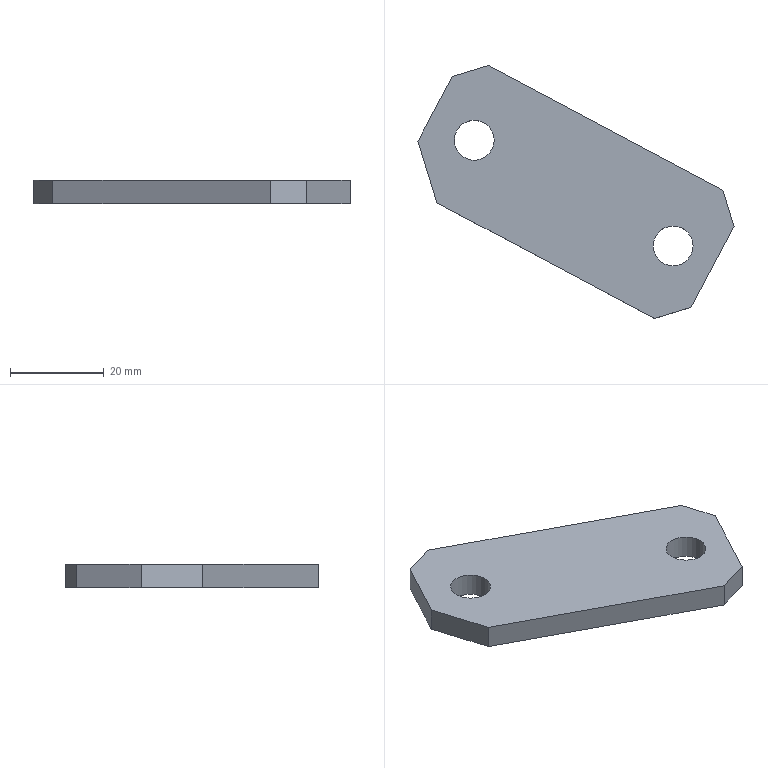Part | STEP file | gslz 2016.10.28-13_id1682_x_t | 1 solid | 12 faces | box 67.358 x 53.937 x 5 mm | volume 9493 mm3 | plane 10 | cylinder 2 | commonest cylinder face diameters 8.5 x2
STEP:
#1=CARTESIAN_POINT('',(0.,0.,0.));
#2=DIRECTION('',(0.,0.,1.));
#3=DIRECTION('',(1.,0.,0.));
#4=AXIS2_PLACEMENT_3D('',#1,#2,#3);
#5=CARTESIAN_POINT('',(446.195,-230.193,-94.));
#6=VERTEX_POINT('',#5);
#7=CARTESIAN_POINT('',(396.233,-203.628,-94.));
#8=VERTEX_POINT('',#7);
#9=CARTESIAN_POINT('',(-202.815,114.892,-94.));
#10=DIRECTION('',(-0.8829,0.4695,0.));
#11=VECTOR('',#10,1.);
#12=LINE('',#9,#11);
#13=CARTESIAN_POINT('',(-202.815,114.892,-99.));
#14=DIRECTION('',(0.4695,0.8829,0.));
#15=DIRECTION('',(-0.8829,0.4695,0.));
#16=AXIS2_PLACEMENT_3D('',#13,#14,#15);
#17=PLANE('',#16);
#18=CARTESIAN_POINT('',(0.,5.));
#19=DIRECTION('',(1.,0.));
#20=VECTOR('',#19,1.);
#21=LINE('',#18,#20);
#22=(GEOMETRIC_REPRESENTATION_CONTEXT(2)PARAMETRIC_REPRESENTATION_CONTEXT()REPRESENTATION_CONTEXT('',''));
#23=DEFINITIONAL_REPRESENTATION('',(#21),#22);
#24=PCURVE('',#17,#23);
#25=CARTESIAN_POINT('',(-224.645,73.835,-94.));
#26=DIRECTION('',(0.,0.,-1.));
#27=DIRECTION('',(-1.,0.,0.));
#28=AXIS2_PLACEMENT_3D('',#25,#26,#27);
#29=PLANE('',#28);
#30=CARTESIAN_POINT('',(-21.83,41.057));
#31=DIRECTION('',(0.8829,0.4695));
#32=VECTOR('',#31,1.);
#33=LINE('',#30,#32);
#34=(GEOMETRIC_REPRESENTATION_CONTEXT(2)PARAMETRIC_REPRESENTATION_CONTEXT()REPRESENTATION_CONTEXT('',''));
#35=DEFINITIONAL_REPRESENTATION('',(#33),#34);
#36=PCURVE('',#29,#35);
#37=SURFACE_CURVE('',#12,(#24,#36),.PCURVE_S1.);
#38=EDGE_CURVE('',#6,#8,#37,.T.);
#39=ORIENTED_EDGE('',*,*,#38,.F.);
#40=CARTESIAN_POINT('',(446.195,-230.193,-99.));
#41=VERTEX_POINT('',#40);
#42=CARTESIAN_POINT('',(446.195,-230.193,-99.));
#43=DIRECTION('',(0.,0.,-1.));
#44=VECTOR('',#43,1.);
#45=LINE('',#42,#44);
#46=CARTESIAN_POINT('',(-735.049,0.));
#47=DIRECTION('',(0.,-1.));
#48=VECTOR('',#47,1.);
#49=LINE('',#46,#48);
#50=(GEOMETRIC_REPRESENTATION_CONTEXT(2)PARAMETRIC_REPRESENTATION_CONTEXT()REPRESENTATION_CONTEXT('',''));
#51=DEFINITIONAL_REPRESENTATION('',(#49),#50);
#52=PCURVE('',#17,#51);
#53=CARTESIAN_POINT('',(448.615,-238.11,-99.));
#54=DIRECTION('',(-0.9563,-0.2924,0.));
#55=DIRECTION('',(0.,0.,1.));
#56=AXIS2_PLACEMENT_3D('',#53,#54,#55);
#57=PLANE('',#56);
#58=CARTESIAN_POINT('',(0.,8.278));
#59=DIRECTION('',(-1.,0.));
#60=VECTOR('',#59,1.);
#61=LINE('',#58,#60);
#62=(GEOMETRIC_REPRESENTATION_CONTEXT(2)PARAMETRIC_REPRESENTATION_CONTEXT()REPRESENTATION_CONTEXT('',''));
#63=DEFINITIONAL_REPRESENTATION('',(#61),#62);
#64=PCURVE('',#57,#63);
#65=SURFACE_CURVE('',#45,(#52,#64),.PCURVE_S1.);
#66=EDGE_CURVE('',#6,#41,#65,.T.);
#67=ORIENTED_EDGE('',*,*,#66,.T.);
#68=CARTESIAN_POINT('',(396.233,-203.628,-99.));
#69=VERTEX_POINT('',#68);
#70=CARTESIAN_POINT('',(-202.815,114.892,-99.));
#71=DIRECTION('',(-0.8829,0.4695,0.));
#72=VECTOR('',#71,1.);
#73=LINE('',#70,#72);
#74=CARTESIAN_POINT('',(0.,0.));
#75=DIRECTION('',(1.,0.));
#76=VECTOR('',#75,1.);
#77=LINE('',#74,#76);
#78=(GEOMETRIC_REPRESENTATION_CONTEXT(2)PARAMETRIC_REPRESENTATION_CONTEXT()REPRESENTATION_CONTEXT('',''));
#79=DEFINITIONAL_REPRESENTATION('',(#77),#78);
#80=PCURVE('',#17,#79);
#81=CARTESIAN_POINT('',(-224.645,73.835,-99.));
#82=DIRECTION('',(0.,0.,-1.));
#83=DIRECTION('',(-1.,0.,0.));
#84=AXIS2_PLACEMENT_3D('',#81,#82,#83);
#85=PLANE('',#84);
#86=CARTESIAN_POINT('',(-21.83,41.057));
#87=DIRECTION('',(0.8829,0.4695));
#88=VECTOR('',#87,1.);
#89=LINE('',#86,#88);
#90=(GEOMETRIC_REPRESENTATION_CONTEXT(2)PARAMETRIC_REPRESENTATION_CONTEXT()REPRESENTATION_CONTEXT('',''));
#91=DEFINITIONAL_REPRESENTATION('',(#89),#90);
#92=PCURVE('',#85,#91);
#93=SURFACE_CURVE('',#73,(#80,#92),.PCURVE_S1.);
#94=EDGE_CURVE('',#41,#69,#93,.T.);
#95=ORIENTED_EDGE('',*,*,#94,.T.);
#96=CARTESIAN_POINT('',(396.233,-203.628,-99.));
#97=DIRECTION('',(0.,0.,1.));
#98=VECTOR('',#97,1.);
#99=LINE('',#96,#98);
#100=CARTESIAN_POINT('',(-678.463,0.));
#101=DIRECTION('',(0.,1.));
#102=VECTOR('',#101,1.);
#103=LINE('',#100,#102);
#104=(GEOMETRIC_REPRESENTATION_CONTEXT(2)PARAMETRIC_REPRESENTATION_CONTEXT()REPRESENTATION_CONTEXT('',''));
#105=DEFINITIONAL_REPRESENTATION('',(#103),#104);
#106=PCURVE('',#17,#105);
#107=CARTESIAN_POINT('',(396.431,-203.567,-99.));
#108=DIRECTION('',(-0.2924,0.9563,0.));
#109=DIRECTION('',(0.,0.,-1.));
#110=AXIS2_PLACEMENT_3D('',#107,#108,#109);
#111=PLANE('',#110);
#112=CARTESIAN_POINT('',(0.,0.2071));
#113=DIRECTION('',(-1.,0.));
#114=VECTOR('',#113,1.);
#115=LINE('',#112,#114);
#116=(GEOMETRIC_REPRESENTATION_CONTEXT(2)PARAMETRIC_REPRESENTATION_CONTEXT()REPRESENTATION_CONTEXT('',''));
#117=DEFINITIONAL_REPRESENTATION('',(#115),#116);
#118=PCURVE('',#111,#117);
#119=SURFACE_CURVE('',#99,(#106,#118),.PCURVE_S1.);
#120=EDGE_CURVE('',#69,#8,#119,.T.);
#121=ORIENTED_EDGE('',*,*,#120,.T.);
#122=EDGE_LOOP('',(#39,#67,#95,#121));
#123=FACE_BOUND('',#122,.T.);
#124=ADVANCED_FACE('',(#123),#17,.T.);
#125=CARTESIAN_POINT('',(439.36,-255.205,-94.));
#126=VERTEX_POINT('',#125);
#127=CARTESIAN_POINT('',(448.555,-237.912,-94.));
#128=VERTEX_POINT('',#127);
#129=CARTESIAN_POINT('',(429.404,-273.93,-94.));
#130=DIRECTION('',(0.4695,0.8829,0.));
#131=VECTOR('',#130,1.);
#132=LINE('',#129,#131);
#133=CARTESIAN_POINT('',(429.404,-273.93,-99.));
#134=DIRECTION('',(0.8829,-0.4695,0.));
#135=DIRECTION('',(0.4695,0.8829,0.));
#136=AXIS2_PLACEMENT_3D('',#133,#134,#135);
#137=PLANE('',#136);
#138=CARTESIAN_POINT('',(0.,5.));
#139=DIRECTION('',(1.,0.));
#140=VECTOR('',#139,1.);
#141=LINE('',#138,#140);
#142=(GEOMETRIC_REPRESENTATION_CONTEXT(2)PARAMETRIC_REPRESENTATION_CONTEXT()REPRESENTATION_CONTEXT('',''));
#143=DEFINITIONAL_REPRESENTATION('',(#141),#142);
#144=PCURVE('',#137,#143);
#145=CARTESIAN_POINT('',(-654.049,-347.764));
#146=DIRECTION('',(-0.4695,0.8829));
#147=VECTOR('',#146,1.);
#148=LINE('',#145,#147);
#149=(GEOMETRIC_REPRESENTATION_CONTEXT(2)PARAMETRIC_REPRESENTATION_CONTEXT()REPRESENTATION_CONTEXT('',''));
#150=DEFINITIONAL_REPRESENTATION('',(#148),#149);
#151=PCURVE('',#29,#150);
#152=SURFACE_CURVE('',#132,(#144,#151),.PCURVE_S1.);
#153=EDGE_CURVE('',#126,#128,#152,.T.);
#154=ORIENTED_EDGE('',*,*,#153,.F.);
#155=CARTESIAN_POINT('',(439.36,-255.205,-99.));
#156=VERTEX_POINT('',#155);
#157=CARTESIAN_POINT('',(439.36,-255.205,-99.));
#158=DIRECTION('',(0.,0.,-1.));
#159=VECTOR('',#158,1.);
#160=LINE('',#157,#159);
#161=CARTESIAN_POINT('',(21.207,0.));
#162=DIRECTION('',(0.,-1.));
#163=VECTOR('',#162,1.);
#164=LINE('',#161,#163);
#165=(GEOMETRIC_REPRESENTATION_CONTEXT(2)PARAMETRIC_REPRESENTATION_CONTEXT()REPRESENTATION_CONTEXT('',''));
#166=DEFINITIONAL_REPRESENTATION('',(#164),#165);
#167=PCURVE('',#137,#166);
#168=CARTESIAN_POINT('',(431.443,-257.625,-99.));
#169=DIRECTION('',(0.2924,-0.9563,0.));
#170=DIRECTION('',(0.,0.,-1.));
#171=AXIS2_PLACEMENT_3D('',#168,#169,#170);
#172=PLANE('',#171);
#173=CARTESIAN_POINT('',(0.,8.278));
#174=DIRECTION('',(1.,0.));
#175=VECTOR('',#174,1.);
#176=LINE('',#173,#175);
#177=(GEOMETRIC_REPRESENTATION_CONTEXT(2)PARAMETRIC_REPRESENTATION_CONTEXT()REPRESENTATION_CONTEXT('',''));
#178=DEFINITIONAL_REPRESENTATION('',(#176),#177);
#179=PCURVE('',#172,#178);
#180=SURFACE_CURVE('',#160,(#167,#179),.PCURVE_S1.);
#181=EDGE_CURVE('',#126,#156,#180,.T.);
#182=ORIENTED_EDGE('',*,*,#181,.T.);
#183=CARTESIAN_POINT('',(448.555,-237.912,-99.));
#184=VERTEX_POINT('',#183);
#185=CARTESIAN_POINT('',(429.404,-273.93,-99.));
#186=DIRECTION('',(0.4695,0.8829,0.));
#187=VECTOR('',#186,1.);
#188=LINE('',#185,#187);
#189=CARTESIAN_POINT('',(0.,0.));
#190=DIRECTION('',(1.,0.));
#191=VECTOR('',#190,1.);
#192=LINE('',#189,#191);
#193=(GEOMETRIC_REPRESENTATION_CONTEXT(2)PARAMETRIC_REPRESENTATION_CONTEXT()REPRESENTATION_CONTEXT('',''));
#194=DEFINITIONAL_REPRESENTATION('',(#192),#193);
#195=PCURVE('',#137,#194);
#196=CARTESIAN_POINT('',(-654.049,-347.764));
#197=DIRECTION('',(-0.4695,0.8829));
#198=VECTOR('',#197,1.);
#199=LINE('',#196,#198);
#200=(GEOMETRIC_REPRESENTATION_CONTEXT(2)PARAMETRIC_REPRESENTATION_CONTEXT()REPRESENTATION_CONTEXT('',''));
#201=DEFINITIONAL_REPRESENTATION('',(#199),#200);
#202=PCURVE('',#85,#201);
#203=SURFACE_CURVE('',#188,(#195,#202),.PCURVE_S1.);
#204=EDGE_CURVE('',#156,#184,#203,.T.);
#205=ORIENTED_EDGE('',*,*,#204,.T.);
#206=CARTESIAN_POINT('',(448.555,-237.912,-99.));
#207=DIRECTION('',(0.,0.,1.));
#208=VECTOR('',#207,1.);
#209=LINE('',#206,#208);
#210=CARTESIAN_POINT('',(40.793,0.));
#211=DIRECTION('',(0.,1.));
#212=VECTOR('',#211,1.);
#213=LINE('',#210,#212);
#214=(GEOMETRIC_REPRESENTATION_CONTEXT(2)PARAMETRIC_REPRESENTATION_CONTEXT()REPRESENTATION_CONTEXT('',''));
#215=DEFINITIONAL_REPRESENTATION('',(#213),#214);
#216=PCURVE('',#137,#215);
#217=CARTESIAN_POINT('',(0.,0.2071));
#218=DIRECTION('',(1.,0.));
#219=VECTOR('',#218,1.);
#220=LINE('',#217,#219);
#221=(GEOMETRIC_REPRESENTATION_CONTEXT(2)PARAMETRIC_REPRESENTATION_CONTEXT()REPRESENTATION_CONTEXT('',''));
#222=DEFINITIONAL_REPRESENTATION('',(#220),#221);
#223=PCURVE('',#57,#222);
#224=SURFACE_CURVE('',#209,(#216,#223),.PCURVE_S1.);
#225=EDGE_CURVE('',#184,#128,#224,.T.);
#226=ORIENTED_EDGE('',*,*,#225,.T.);
#227=EDGE_LOOP('',(#154,#182,#205,#226));
#228=FACE_BOUND('',#227,.T.);
#229=ADVANCED_FACE('',(#228),#137,.T.);
#230=CARTESIAN_POINT('',(431.641,-257.564,-94.));
#231=VERTEX_POINT('',#230);
#232=CARTESIAN_POINT('',(385.211,-232.877,-94.));
#233=VERTEX_POINT('',#232);
#234=CARTESIAN_POINT('',(-217.368,87.52,-94.));
#235=DIRECTION('',(-0.8829,0.4695,0.));
#236=VECTOR('',#235,1.);
#237=LINE('',#234,#236);
#238=CARTESIAN_POINT('',(-217.368,87.52,-99.));
#239=DIRECTION('',(0.4695,0.8829,0.));
#240=DIRECTION('',(-0.8829,0.4695,0.));
#241=AXIS2_PLACEMENT_3D('',#238,#239,#240);
#242=PLANE('',#241);
#243=CARTESIAN_POINT('',(0.,5.));
#244=DIRECTION('',(1.,0.));
#245=VECTOR('',#244,1.);
#246=LINE('',#243,#245);
#247=(GEOMETRIC_REPRESENTATION_CONTEXT(2)PARAMETRIC_REPRESENTATION_CONTEXT()REPRESENTATION_CONTEXT('',''));
#248=DEFINITIONAL_REPRESENTATION('',(#246),#247);
#249=PCURVE('',#242,#248);
#250=CARTESIAN_POINT('',(-7.277,13.686));
#251=DIRECTION('',(0.8829,0.4695));
#252=VECTOR('',#251,1.);
#253=LINE('',#250,#252);
#254=(GEOMETRIC_REPRESENTATION_CONTEXT(2)PARAMETRIC_REPRESENTATION_CONTEXT()REPRESENTATION_CONTEXT('',''));
#255=DEFINITIONAL_REPRESENTATION('',(#253),#254);
#256=PCURVE('',#29,#255);
#257=SURFACE_CURVE('',#237,(#249,#256),.PCURVE_S1.);
#258=EDGE_CURVE('',#231,#233,#257,.T.);
#259=ORIENTED_EDGE('',*,*,#258,.T.);
#260=CARTESIAN_POINT('',(385.211,-232.877,-99.));
#261=VERTEX_POINT('',#260);
#262=CARTESIAN_POINT('',(385.211,-232.877,-99.));
#263=DIRECTION('',(0.,0.,-1.));
#264=VECTOR('',#263,1.);
#265=LINE('',#262,#264);
#266=CARTESIAN_POINT('',(-682.463,0.));
#267=DIRECTION('',(0.,-1.));
#268=VECTOR('',#267,1.);
#269=LINE('',#266,#268);
#270=(GEOMETRIC_REPRESENTATION_CONTEXT(2)PARAMETRIC_REPRESENTATION_CONTEXT()REPRESENTATION_CONTEXT('',''));
#271=DEFINITIONAL_REPRESENTATION('',(#269),#270);
#272=PCURVE('',#242,#271);
#273=CARTESIAN_POINT('',(381.137,-219.551,-99.));
#274=DIRECTION('',(0.9563,0.2924,0.));
#275=DIRECTION('',(0.,0.,1.));
#276=AXIS2_PLACEMENT_3D('',#273,#274,#275);
#277=PLANE('',#276);
#278=CARTESIAN_POINT('',(0.,13.935));
#279=DIRECTION('',(-1.,0.));
#280=VECTOR('',#279,1.);
#281=LINE('',#278,#280);
#282=(GEOMETRIC_REPRESENTATION_CONTEXT(2)PARAMETRIC_REPRESENTATION_CONTEXT()REPRESENTATION_CONTEXT('',''));
#283=DEFINITIONAL_REPRESENTATION('',(#281),#282);
#284=PCURVE('',#277,#283);
#285=SURFACE_CURVE('',#265,(#272,#284),.PCURVE_S1.);
#286=EDGE_CURVE('',#233,#261,#285,.T.);
#287=ORIENTED_EDGE('',*,*,#286,.T.);
#288=CARTESIAN_POINT('',(431.641,-257.564,-99.));
#289=VERTEX_POINT('',#288);
#290=CARTESIAN_POINT('',(-217.368,87.52,-99.));
#291=DIRECTION('',(-0.8829,0.4695,0.));
#292=VECTOR('',#291,1.);
#293=LINE('',#290,#292);
#294=CARTESIAN_POINT('',(0.,0.));
#295=DIRECTION('',(1.,0.));
#296=VECTOR('',#295,1.);
#297=LINE('',#294,#296);
#298=(GEOMETRIC_REPRESENTATION_CONTEXT(2)PARAMETRIC_REPRESENTATION_CONTEXT()REPRESENTATION_CONTEXT('',''));
#299=DEFINITIONAL_REPRESENTATION('',(#297),#298);
#300=PCURVE('',#242,#299);
#301=CARTESIAN_POINT('',(-7.277,13.686));
#302=DIRECTION('',(0.8829,0.4695));
#303=VECTOR('',#302,1.);
#304=LINE('',#301,#303);
#305=(GEOMETRIC_REPRESENTATION_CONTEXT(2)PARAMETRIC_REPRESENTATION_CONTEXT()REPRESENTATION_CONTEXT('',''));
#306=DEFINITIONAL_REPRESENTATION('',(#304),#305);
#307=PCURVE('',#85,#306);
#308=SURFACE_CURVE('',#293,(#300,#307),.PCURVE_S1.);
#309=EDGE_CURVE('',#289,#261,#308,.T.);
#310=ORIENTED_EDGE('',*,*,#309,.F.);
#311=CARTESIAN_POINT('',(431.641,-257.564,-99.));
#312=DIRECTION('',(0.,0.,1.));
#313=VECTOR('',#312,1.);
#314=LINE('',#311,#313);
#315=CARTESIAN_POINT('',(-735.049,0.));
#316=DIRECTION('',(0.,1.));
#317=VECTOR('',#316,1.);
#318=LINE('',#315,#317);
#319=(GEOMETRIC_REPRESENTATION_CONTEXT(2)PARAMETRIC_REPRESENTATION_CONTEXT()REPRESENTATION_CONTEXT('',''));
#320=DEFINITIONAL_REPRESENTATION('',(#318),#319);
#321=PCURVE('',#242,#320);
#322=CARTESIAN_POINT('',(0.,0.2071));
#323=DIRECTION('',(-1.,0.));
#324=VECTOR('',#323,1.);
#325=LINE('',#322,#324);
#326=(GEOMETRIC_REPRESENTATION_CONTEXT(2)PARAMETRIC_REPRESENTATION_CONTEXT()REPRESENTATION_CONTEXT('',''));
#327=DEFINITIONAL_REPRESENTATION('',(#325),#326);
#328=PCURVE('',#172,#327);
#329=SURFACE_CURVE('',#314,(#321,#328),.PCURVE_S1.);
#330=EDGE_CURVE('',#289,#231,#329,.T.);
#331=ORIENTED_EDGE('',*,*,#330,.T.);
#332=EDGE_LOOP('',(#259,#287,#310,#331));
#333=FACE_BOUND('',#332,.T.);
#334=ADVANCED_FACE('',(#333),#242,.F.);
#335=CARTESIAN_POINT('',(431.319,-242.098,-99.));
#336=VERTEX_POINT('',#335);
#337=CARTESIAN_POINT('',(435.569,-242.098,-99.));
#338=DIRECTION('',(0.,0.,-1.));
#339=DIRECTION('',(-1.,0.,0.));
#340=AXIS2_PLACEMENT_3D('',#337,#338,#339);
#341=CIRCLE('',#340,4.25);
#342=CARTESIAN_POINT('',(435.569,-242.098,-99.));
#343=DIRECTION('',(0.,0.,1.));
#344=DIRECTION('',(1.,0.,0.));
#345=AXIS2_PLACEMENT_3D('',#342,#343,#344);
#346=CYLINDRICAL_SURFACE('',#345,4.25);
#347=CARTESIAN_POINT('',(9.425,0.));
#348=DIRECTION('',(-1.,0.));
#349=VECTOR('',#348,1.);
#350=LINE('',#347,#349);
#351=(GEOMETRIC_REPRESENTATION_CONTEXT(2)PARAMETRIC_REPRESENTATION_CONTEXT()REPRESENTATION_CONTEXT('',''));
#352=DEFINITIONAL_REPRESENTATION('',(#350),#351);
#353=PCURVE('',#346,#352);
#354=CARTESIAN_POINT('',(-660.215,-315.933));
#355=DIRECTION('',(1.,0.));
#356=AXIS2_PLACEMENT_2D('',#354,#355);
#357=CIRCLE('',#356,4.25);
#358=(GEOMETRIC_REPRESENTATION_CONTEXT(2)PARAMETRIC_REPRESENTATION_CONTEXT()REPRESENTATION_CONTEXT('',''));
#359=DEFINITIONAL_REPRESENTATION('',(#357),#358);
#360=PCURVE('',#85,#359);
#361=SURFACE_CURVE('',#341,(#353,#360),.PCURVE_S1.);
#362=EDGE_CURVE('',#336,#336,#361,.T.);
#363=ORIENTED_EDGE('',*,*,#362,.F.);
#364=CARTESIAN_POINT('',(431.319,-242.098,-94.));
#365=VERTEX_POINT('',#364);
#366=CARTESIAN_POINT('',(431.319,-242.098,-99.));
#367=CARTESIAN_POINT('',(431.319,-242.098,-94.));
#368=B_SPLINE_CURVE_WITH_KNOTS('',1,(#366,#367),.UNSPECIFIED.,.F.,.F.,(2,2),(0.,5.),.PIECEWISE_BEZIER_KNOTS.);
#369=CARTESIAN_POINT('',(9.425,0.));
#370=DIRECTION('',(0.,1.));
#371=VECTOR('',#370,1.);
#372=LINE('',#369,#371);
#373=(GEOMETRIC_REPRESENTATION_CONTEXT(2)PARAMETRIC_REPRESENTATION_CONTEXT()REPRESENTATION_CONTEXT('',''));
#374=DEFINITIONAL_REPRESENTATION('',(#372),#373);
#375=PCURVE('',#346,#374);
#376=CARTESIAN_POINT('',(3.142,0.));
#377=DIRECTION('',(0.,1.));
#378=VECTOR('',#377,1.);
#379=LINE('',#376,#378);
#380=(GEOMETRIC_REPRESENTATION_CONTEXT(2)PARAMETRIC_REPRESENTATION_CONTEXT()REPRESENTATION_CONTEXT('',''));
#381=DEFINITIONAL_REPRESENTATION('',(#379),#380);
#382=PCURVE('',#346,#381);
#383=SEAM_CURVE('',#368,(#375,#382),.PCURVE_S1.);
#384=EDGE_CURVE('',#336,#365,#383,.T.);
#385=ORIENTED_EDGE('',*,*,#384,.T.);
#386=CARTESIAN_POINT('',(435.569,-242.098,-94.));
#387=DIRECTION('',(0.,0.,-1.));
#388=DIRECTION('',(-1.,0.,0.));
#389=AXIS2_PLACEMENT_3D('',#386,#387,#388);
#390=CIRCLE('',#389,4.25);
#391=CARTESIAN_POINT('',(9.425,5.));
#392=DIRECTION('',(-1.,0.));
#393=VECTOR('',#392,1.);
#394=LINE('',#391,#393);
#395=(GEOMETRIC_REPRESENTATION_CONTEXT(2)PARAMETRIC_REPRESENTATION_CONTEXT()REPRESENTATION_CONTEXT('',''));
#396=DEFINITIONAL_REPRESENTATION('',(#394),#395);
#397=PCURVE('',#346,#396);
#398=CARTESIAN_POINT('',(-660.215,-315.933));
#399=DIRECTION('',(1.,0.));
#400=AXIS2_PLACEMENT_2D('',#398,#399);
#401=CIRCLE('',#400,4.25);
#402=(GEOMETRIC_REPRESENTATION_CONTEXT(2)PARAMETRIC_REPRESENTATION_CONTEXT()REPRESENTATION_CONTEXT('',''));
#403=DEFINITIONAL_REPRESENTATION('',(#401),#402);
#404=PCURVE('',#29,#403);
#405=SURFACE_CURVE('',#390,(#397,#404),.PCURVE_S1.);
#406=EDGE_CURVE('',#365,#365,#405,.T.);
#407=ORIENTED_EDGE('',*,*,#406,.T.);
#408=ORIENTED_EDGE('',*,*,#384,.F.);
#409=EDGE_LOOP('',(#363,#385,#407,#408));
#410=FACE_BOUND('',#409,.F.);
#411=ADVANCED_FACE('',(#410),#346,.F.);
#412=CARTESIAN_POINT('',(388.938,-219.564,-99.));
#413=VERTEX_POINT('',#412);
#414=CARTESIAN_POINT('',(393.188,-219.564,-99.));
#415=DIRECTION('',(0.,0.,-1.));
#416=DIRECTION('',(-1.,0.,0.));
#417=AXIS2_PLACEMENT_3D('',#414,#415,#416);
#418=CIRCLE('',#417,4.25);
#419=CARTESIAN_POINT('',(393.188,-219.564,-99.));
#420=DIRECTION('',(0.,0.,1.));
#421=DIRECTION('',(1.,0.,0.));
#422=AXIS2_PLACEMENT_3D('',#419,#420,#421);
#423=CYLINDRICAL_SURFACE('',#422,4.25);
#424=CARTESIAN_POINT('',(9.425,0.));
#425=DIRECTION('',(-1.,0.));
#426=VECTOR('',#425,1.);
#427=LINE('',#424,#426);
#428=(GEOMETRIC_REPRESENTATION_CONTEXT(2)PARAMETRIC_REPRESENTATION_CONTEXT()REPRESENTATION_CONTEXT('',''));
#429=DEFINITIONAL_REPRESENTATION('',(#427),#428);
#430=PCURVE('',#423,#429);
#431=CARTESIAN_POINT('',(-617.833,-293.398));
#432=DIRECTION('',(1.,0.));
#433=AXIS2_PLACEMENT_2D('',#431,#432);
#434=CIRCLE('',#433,4.25);
#435=(GEOMETRIC_REPRESENTATION_CONTEXT(2)PARAMETRIC_REPRESENTATION_CONTEXT()REPRESENTATION_CONTEXT('',''));
#436=DEFINITIONAL_REPRESENTATION('',(#434),#435);
#437=PCURVE('',#85,#436);
#438=SURFACE_CURVE('',#418,(#430,#437),.PCURVE_S1.);
#439=EDGE_CURVE('',#413,#413,#438,.T.);
#440=ORIENTED_EDGE('',*,*,#439,.F.);
#441=CARTESIAN_POINT('',(388.938,-219.564,-94.));
#442=VERTEX_POINT('',#441);
#443=CARTESIAN_POINT('',(388.938,-219.564,-99.));
#444=CARTESIAN_POINT('',(388.938,-219.564,-94.));
#445=B_SPLINE_CURVE_WITH_KNOTS('',1,(#443,#444),.UNSPECIFIED.,.F.,.F.,(2,2),(0.,5.),.PIECEWISE_BEZIER_KNOTS.);
#446=CARTESIAN_POINT('',(9.425,0.));
#447=DIRECTION('',(0.,1.));
#448=VECTOR('',#447,1.);
#449=LINE('',#446,#448);
#450=(GEOMETRIC_REPRESENTATION_CONTEXT(2)PARAMETRIC_REPRESENTATION_CONTEXT()REPRESENTATION_CONTEXT('',''));
#451=DEFINITIONAL_REPRESENTATION('',(#449),#450);
#452=PCURVE('',#423,#451);
#453=CARTESIAN_POINT('',(3.142,0.));
#454=DIRECTION('',(0.,1.));
#455=VECTOR('',#454,1.);
#456=LINE('',#453,#455);
#457=(GEOMETRIC_REPRESENTATION_CONTEXT(2)PARAMETRIC_REPRESENTATION_CONTEXT()REPRESENTATION_CONTEXT('',''));
#458=DEFINITIONAL_REPRESENTATION('',(#456),#457);
#459=PCURVE('',#423,#458);
#460=SEAM_CURVE('',#445,(#452,#459),.PCURVE_S1.);
#461=EDGE_CURVE('',#413,#442,#460,.T.);
#462=ORIENTED_EDGE('',*,*,#461,.T.);
#463=CARTESIAN_POINT('',(393.188,-219.564,-94.));
#464=DIRECTION('',(0.,0.,-1.));
#465=DIRECTION('',(-1.,0.,0.));
#466=AXIS2_PLACEMENT_3D('',#463,#464,#465);
#467=CIRCLE('',#466,4.25);
#468=CARTESIAN_POINT('',(9.425,5.));
#469=DIRECTION('',(-1.,0.));
#470=VECTOR('',#469,1.);
#471=LINE('',#468,#470);
#472=(GEOMETRIC_REPRESENTATION_CONTEXT(2)PARAMETRIC_REPRESENTATION_CONTEXT()REPRESENTATION_CONTEXT('',''));
#473=DEFINITIONAL_REPRESENTATION('',(#471),#472);
#474=PCURVE('',#423,#473);
#475=CARTESIAN_POINT('',(-617.833,-293.398));
#476=DIRECTION('',(1.,0.));
#477=AXIS2_PLACEMENT_2D('',#475,#476);
#478=CIRCLE('',#477,4.25);
#479=(GEOMETRIC_REPRESENTATION_CONTEXT(2)PARAMETRIC_REPRESENTATION_CONTEXT()REPRESENTATION_CONTEXT('',''));
#480=DEFINITIONAL_REPRESENTATION('',(#478),#479);
#481=PCURVE('',#29,#480);
#482=SURFACE_CURVE('',#467,(#474,#481),.PCURVE_S1.);
#483=EDGE_CURVE('',#442,#442,#482,.T.);
#484=ORIENTED_EDGE('',*,*,#483,.T.);
#485=ORIENTED_EDGE('',*,*,#461,.F.);
#486=EDGE_LOOP('',(#440,#462,#484,#485));
#487=FACE_BOUND('',#486,.F.);
#488=ADVANCED_FACE('',(#487),#423,.F.);
#489=CARTESIAN_POINT('',(381.197,-219.749,-99.));
#490=VERTEX_POINT('',#489);
#491=CARTESIAN_POINT('',(388.514,-205.987,-99.));
#492=VERTEX_POINT('',#491);
#493=CARTESIAN_POINT('',(369.363,-242.005,-99.));
#494=DIRECTION('',(0.4695,0.8829,0.));
#495=VECTOR('',#494,1.);
#496=LINE('',#493,#495);
#497=CARTESIAN_POINT('',(369.363,-242.005,-99.));
#498=DIRECTION('',(0.8829,-0.4695,0.));
#499=DIRECTION('',(0.4695,0.8829,0.));
#500=AXIS2_PLACEMENT_3D('',#497,#498,#499);
#501=PLANE('',#500);
#502=CARTESIAN_POINT('',(0.,0.));
#503=DIRECTION('',(1.,0.));
#504=VECTOR('',#503,1.);
#505=LINE('',#502,#504);
#506=(GEOMETRIC_REPRESENTATION_CONTEXT(2)PARAMETRIC_REPRESENTATION_CONTEXT()REPRESENTATION_CONTEXT('',''));
#507=DEFINITIONAL_REPRESENTATION('',(#505),#506);
#508=PCURVE('',#501,#507);
#509=CARTESIAN_POINT('',(-594.009,-315.84));
#510=DIRECTION('',(-0.4695,0.8829));
#511=VECTOR('',#510,1.);
#512=LINE('',#509,#511);
#513=(GEOMETRIC_REPRESENTATION_CONTEXT(2)PARAMETRIC_REPRESENTATION_CONTEXT()REPRESENTATION_CONTEXT('',''));
#514=DEFINITIONAL_REPRESENTATION('',(#512),#513);
#515=PCURVE('',#85,#514);
#516=SURFACE_CURVE('',#496,(#508,#515),.PCURVE_S1.);
#517=EDGE_CURVE('',#490,#492,#516,.T.);
#518=ORIENTED_EDGE('',*,*,#517,.F.);
#519=CARTESIAN_POINT('',(381.197,-219.749,-94.));
#520=VERTEX_POINT('',#519);
#521=CARTESIAN_POINT('',(381.197,-219.749,-99.));
#522=DIRECTION('',(0.,0.,1.));
#523=VECTOR('',#522,1.);
#524=LINE('',#521,#523);
#525=CARTESIAN_POINT('',(25.207,0.));
#526=DIRECTION('',(0.,1.));
#527=VECTOR('',#526,1.);
#528=LINE('',#525,#527);
#529=(GEOMETRIC_REPRESENTATION_CONTEXT(2)PARAMETRIC_REPRESENTATION_CONTEXT()REPRESENTATION_CONTEXT('',''));
#530=DEFINITIONAL_REPRESENTATION('',(#528),#529);
#531=PCURVE('',#501,#530);
#532=CARTESIAN_POINT('',(0.,0.2071));
#533=DIRECTION('',(1.,0.));
#534=VECTOR('',#533,1.);
#535=LINE('',#532,#534);
#536=(GEOMETRIC_REPRESENTATION_CONTEXT(2)PARAMETRIC_REPRESENTATION_CONTEXT()REPRESENTATION_CONTEXT('',''));
#537=DEFINITIONAL_REPRESENTATION('',(#535),#536);
#538=PCURVE('',#277,#537);
#539=SURFACE_CURVE('',#524,(#531,#538),.PCURVE_S1.);
#540=EDGE_CURVE('',#490,#520,#539,.T.);
#541=ORIENTED_EDGE('',*,*,#540,.T.);
#542=CARTESIAN_POINT('',(388.514,-205.987,-94.));
#543=VERTEX_POINT('',#542);
#544=CARTESIAN_POINT('',(369.363,-242.005,-94.));
#545=DIRECTION('',(0.4695,0.8829,0.));
#546=VECTOR('',#545,1.);
#547=LINE('',#544,#546);
#548=CARTESIAN_POINT('',(0.,5.));
#549=DIRECTION('',(1.,0.));
#550=VECTOR('',#549,1.);
#551=LINE('',#548,#550);
#552=(GEOMETRIC_REPRESENTATION_CONTEXT(2)PARAMETRIC_REPRESENTATION_CONTEXT()REPRESENTATION_CONTEXT('',''));
#553=DEFINITIONAL_REPRESENTATION('',(#551),#552);
#554=PCURVE('',#501,#553);
#555=CARTESIAN_POINT('',(-594.009,-315.84));
#556=DIRECTION('',(-0.4695,0.8829));
#557=VECTOR('',#556,1.);
#558=LINE('',#555,#557);
#559=(GEOMETRIC_REPRESENTATION_CONTEXT(2)PARAMETRIC_REPRESENTATION_CONTEXT()REPRESENTATION_CONTEXT('',''));
#560=DEFINITIONAL_REPRESENTATION('',(#558),#559);
#561=PCURVE('',#29,#560);
#562=SURFACE_CURVE('',#547,(#554,#561),.PCURVE_S1.);
#563=EDGE_CURVE('',#520,#543,#562,.T.);
#564=ORIENTED_EDGE('',*,*,#563,.T.);
#565=CARTESIAN_POINT('',(388.514,-205.987,-99.));
#566=DIRECTION('',(0.,0.,-1.));
#567=VECTOR('',#566,1.);
#568=LINE('',#565,#567);
#569=CARTESIAN_POINT('',(40.793,0.));
#570=DIRECTION('',(0.,-1.));
#571=VECTOR('',#570,1.);
#572=LINE('',#569,#571);
#573=(GEOMETRIC_REPRESENTATION_CONTEXT(2)PARAMETRIC_REPRESENTATION_CONTEXT()REPRESENTATION_CONTEXT('',''));
#574=DEFINITIONAL_REPRESENTATION('',(#572),#573);
#575=PCURVE('',#501,#574);
#576=CARTESIAN_POINT('',(0.,8.278));
#577=DIRECTION('',(1.,0.));
#578=VECTOR('',#577,1.);
#579=LINE('',#576,#578);
#580=(GEOMETRIC_REPRESENTATION_CONTEXT(2)PARAMETRIC_REPRESENTATION_CONTEXT()REPRESENTATION_CONTEXT('',''));
#581=DEFINITIONAL_REPRESENTATION('',(#579),#580);
#582=PCURVE('',#111,#581);
#583=SURFACE_CURVE('',#568,(#575,#582),.PCURVE_S1.);
#584=EDGE_CURVE('',#543,#492,#583,.T.);
#585=ORIENTED_EDGE('',*,*,#584,.T.);
#586=EDGE_LOOP('',(#518,#541,#564,#585));
#587=FACE_BOUND('',#586,.T.);
#588=ADVANCED_FACE('',(#587),#501,.F.);
#589=ORIENTED_EDGE('',*,*,#439,.F.);
#590=EDGE_LOOP('',(#589));
#591=FACE_BOUND('',#590,.T.);
#592=ORIENTED_EDGE('',*,*,#362,.F.);
#593=EDGE_LOOP('',(#592));
#594=FACE_BOUND('',#593,.T.);
#595=ORIENTED_EDGE('',*,*,#309,.T.);
#596=CARTESIAN_POINT('',(247.324,218.13,-99.));
#597=DIRECTION('',(-0.2924,0.9563,0.));
#598=VECTOR('',#597,1.);
#599=LINE('',#596,#598);
#600=CARTESIAN_POINT('',(-471.97,144.295));
#601=DIRECTION('',(0.2924,0.9563));
#602=VECTOR('',#601,1.);
#603=LINE('',#600,#602);
#604=(GEOMETRIC_REPRESENTATION_CONTEXT(2)PARAMETRIC_REPRESENTATION_CONTEXT()REPRESENTATION_CONTEXT('',''));
#605=DEFINITIONAL_REPRESENTATION('',(#603),#604);
#606=PCURVE('',#85,#605);
#607=CARTESIAN_POINT('',(0.,-457.679));
#608=DIRECTION('',(0.,-1.));
#609=VECTOR('',#608,1.);
#610=LINE('',#607,#609);
#611=(GEOMETRIC_REPRESENTATION_CONTEXT(2)PARAMETRIC_REPRESENTATION_CONTEXT()REPRESENTATION_CONTEXT('',''));
#612=DEFINITIONAL_REPRESENTATION('',(#610),#611);
#613=PCURVE('',#277,#612);
#614=SURFACE_CURVE('',#599,(#606,#613),.PCURVE_S1.);
#615=EDGE_CURVE('',#261,#490,#614,.T.);
#616=ORIENTED_EDGE('',*,*,#615,.T.);
#617=ORIENTED_EDGE('',*,*,#517,.T.);
#618=CARTESIAN_POINT('',(-91.966,-352.885,-99.));
#619=DIRECTION('',(0.9563,0.2924,0.));
#620=VECTOR('',#619,1.);
#621=LINE('',#618,#620);
#622=CARTESIAN_POINT('',(-132.679,-426.72));
#623=DIRECTION('',(-0.9563,0.2924));
#624=VECTOR('',#623,1.);
#625=LINE('',#622,#624);
#626=(GEOMETRIC_REPRESENTATION_CONTEXT(2)PARAMETRIC_REPRESENTATION_CONTEXT()REPRESENTATION_CONTEXT('',''));
#627=DEFINITIONAL_REPRESENTATION('',(#625),#626);
#628=PCURVE('',#85,#627);
#629=CARTESIAN_POINT('',(0.,510.712));
#630=DIRECTION('',(0.,-1.));
#631=VECTOR('',#630,1.);
#632=LINE('',#629,#631);
#633=(GEOMETRIC_REPRESENTATION_CONTEXT(2)PARAMETRIC_REPRESENTATION_CONTEXT()REPRESENTATION_CONTEXT('',''));
#634=DEFINITIONAL_REPRESENTATION('',(#632),#633);
#635=PCURVE('',#111,#634);
#636=SURFACE_CURVE('',#621,(#628,#635),.PCURVE_S1.);
#637=EDGE_CURVE('',#492,#69,#636,.T.);
#638=ORIENTED_EDGE('',*,*,#637,.T.);
#639=ORIENTED_EDGE('',*,*,#94,.F.);
#640=CARTESIAN_POINT('',(303.226,237.439,-99.));
#641=DIRECTION('',(0.2924,-0.9563,0.));
#642=VECTOR('',#641,1.);
#643=LINE('',#640,#642);
#644=CARTESIAN_POINT('',(-527.871,163.604));
#645=DIRECTION('',(-0.2924,-0.9563));
#646=VECTOR('',#645,1.);
#647=LINE('',#644,#646);
#648=(GEOMETRIC_REPRESENTATION_CONTEXT(2)PARAMETRIC_REPRESENTATION_CONTEXT()REPRESENTATION_CONTEXT('',''));
#649=DEFINITIONAL_REPRESENTATION('',(#647),#648);
#650=PCURVE('',#85,#649);
#651=CARTESIAN_POINT('',(0.,497.277));
#652=DIRECTION('',(0.,-1.));
#653=VECTOR('',#652,1.);
#654=LINE('',#651,#653);
#655=(GEOMETRIC_REPRESENTATION_CONTEXT(2)PARAMETRIC_REPRESENTATION_CONTEXT()REPRESENTATION_CONTEXT('',''));
#656=DEFINITIONAL_REPRESENTATION('',(#654),#655);
#657=PCURVE('',#57,#656);
#658=SURFACE_CURVE('',#643,(#650,#657),.PCURVE_S1.);
#659=EDGE_CURVE('',#41,#184,#658,.T.);
#660=ORIENTED_EDGE('',*,*,#659,.T.);
#661=ORIENTED_EDGE('',*,*,#204,.F.);
#662=CARTESIAN_POINT('',(-75.887,-412.731,-99.));
#663=DIRECTION('',(-0.9563,-0.2924,0.));
#664=VECTOR('',#663,1.);
#665=LINE('',#662,#664);
#666=CARTESIAN_POINT('',(-148.758,-486.566));
#667=DIRECTION('',(0.9563,-0.2924));
#668=VECTOR('',#667,1.);
#669=LINE('',#666,#668);
#670=(GEOMETRIC_REPRESENTATION_CONTEXT(2)PARAMETRIC_REPRESENTATION_CONTEXT()REPRESENTATION_CONTEXT('',''));
#671=DEFINITIONAL_REPRESENTATION('',(#669),#670);
#672=PCURVE('',#85,#671);
#673=CARTESIAN_POINT('',(0.,-530.511));
#674=DIRECTION('',(0.,-1.));
#675=VECTOR('',#674,1.);
#676=LINE('',#673,#675);
#677=(GEOMETRIC_REPRESENTATION_CONTEXT(2)PARAMETRIC_REPRESENTATION_CONTEXT()REPRESENTATION_CONTEXT('',''));
#678=DEFINITIONAL_REPRESENTATION('',(#676),#677);
#679=PCURVE('',#172,#678);
#680=SURFACE_CURVE('',#665,(#672,#679),.PCURVE_S1.);
#681=EDGE_CURVE('',#156,#289,#680,.T.);
#682=ORIENTED_EDGE('',*,*,#681,.T.);
#683=EDGE_LOOP('',(#595,#616,#617,#638,#639,#660,#661,#682));
#684=FACE_BOUND('',#683,.T.);
#685=ADVANCED_FACE('',(#591,#594,#684),#85,.T.);
#686=ORIENTED_EDGE('',*,*,#483,.T.);
#687=EDGE_LOOP('',(#686));
#688=FACE_BOUND('',#687,.T.);
#689=ORIENTED_EDGE('',*,*,#406,.T.);
#690=EDGE_LOOP('',(#689));
#691=FACE_BOUND('',#690,.T.);
#692=ORIENTED_EDGE('',*,*,#563,.F.);
#693=CARTESIAN_POINT('',(381.137,-219.551,-94.));
#694=DIRECTION('',(0.2924,-0.9563,0.));
#695=VECTOR('',#694,1.);
#696=LINE('',#693,#695);
#697=CARTESIAN_POINT('',(-605.782,-293.385));
#698=DIRECTION('',(-0.2924,-0.9563));
#699=VECTOR('',#698,1.);
#700=LINE('',#697,#699);
#701=(GEOMETRIC_REPRESENTATION_CONTEXT(2)PARAMETRIC_REPRESENTATION_CONTEXT()REPRESENTATION_CONTEXT('',''));
#702=DEFINITIONAL_REPRESENTATION('',(#700),#701);
#703=PCURVE('',#29,#702);
#704=CARTESIAN_POINT('',(5.,0.));
#705=DIRECTION('',(0.,1.));
#706=VECTOR('',#705,1.);
#707=LINE('',#704,#706);
#708=(GEOMETRIC_REPRESENTATION_CONTEXT(2)PARAMETRIC_REPRESENTATION_CONTEXT()REPRESENTATION_CONTEXT('',''));
#709=DEFINITIONAL_REPRESENTATION('',(#707),#708);
#710=PCURVE('',#277,#709);
#711=SURFACE_CURVE('',#696,(#703,#710),.PCURVE_S1.);
#712=EDGE_CURVE('',#520,#233,#711,.T.);
#713=ORIENTED_EDGE('',*,*,#712,.T.);
#714=ORIENTED_EDGE('',*,*,#258,.F.);
#715=CARTESIAN_POINT('',(431.443,-257.625,-94.));
#716=DIRECTION('',(0.9563,0.2924,0.));
#717=VECTOR('',#716,1.);
#718=LINE('',#715,#717);
#719=CARTESIAN_POINT('',(-656.089,-331.46));
#720=DIRECTION('',(-0.9563,0.2924));
#721=VECTOR('',#720,1.);
#722=LINE('',#719,#721);
#723=(GEOMETRIC_REPRESENTATION_CONTEXT(2)PARAMETRIC_REPRESENTATION_CONTEXT()REPRESENTATION_CONTEXT('',''));
#724=DEFINITIONAL_REPRESENTATION('',(#722),#723);
#725=PCURVE('',#29,#724);
#726=CARTESIAN_POINT('',(-5.,0.));
#727=DIRECTION('',(0.,1.));
#728=VECTOR('',#727,1.);
#729=LINE('',#726,#728);
#730=(GEOMETRIC_REPRESENTATION_CONTEXT(2)PARAMETRIC_REPRESENTATION_CONTEXT()REPRESENTATION_CONTEXT('',''));
#731=DEFINITIONAL_REPRESENTATION('',(#729),#730);
#732=PCURVE('',#172,#731);
#733=SURFACE_CURVE('',#718,(#725,#732),.PCURVE_S1.);
#734=EDGE_CURVE('',#231,#126,#733,.T.);
#735=ORIENTED_EDGE('',*,*,#734,.T.);
#736=ORIENTED_EDGE('',*,*,#153,.T.);
#737=CARTESIAN_POINT('',(448.615,-238.11,-94.));
#738=DIRECTION('',(-0.2924,0.9563,0.));
#739=VECTOR('',#738,1.);
#740=LINE('',#737,#739);
#741=CARTESIAN_POINT('',(-673.261,-311.944));
#742=DIRECTION('',(0.2924,0.9563));
#743=VECTOR('',#742,1.);
#744=LINE('',#741,#743);
#745=(GEOMETRIC_REPRESENTATION_CONTEXT(2)PARAMETRIC_REPRESENTATION_CONTEXT()REPRESENTATION_CONTEXT('',''));
#746=DEFINITIONAL_REPRESENTATION('',(#744),#745);
#747=PCURVE('',#29,#746);
#748=CARTESIAN_POINT('',(5.,0.));
#749=DIRECTION('',(0.,1.));
#750=VECTOR('',#749,1.);
#751=LINE('',#748,#750);
#752=(GEOMETRIC_REPRESENTATION_CONTEXT(2)PARAMETRIC_REPRESENTATION_CONTEXT()REPRESENTATION_CONTEXT('',''));
#753=DEFINITIONAL_REPRESENTATION('',(#751),#752);
#754=PCURVE('',#57,#753);
#755=SURFACE_CURVE('',#740,(#747,#754),.PCURVE_S1.);
#756=EDGE_CURVE('',#128,#6,#755,.T.);
#757=ORIENTED_EDGE('',*,*,#756,.T.);
#758=ORIENTED_EDGE('',*,*,#38,.T.);
#759=CARTESIAN_POINT('',(396.431,-203.567,-94.));
#760=DIRECTION('',(-0.9563,-0.2924,0.));
#761=VECTOR('',#760,1.);
#762=LINE('',#759,#761);
#763=CARTESIAN_POINT('',(-621.076,-277.402));
#764=DIRECTION('',(0.9563,-0.2924));
#765=VECTOR('',#764,1.);
#766=LINE('',#763,#765);
#767=(GEOMETRIC_REPRESENTATION_CONTEXT(2)PARAMETRIC_REPRESENTATION_CONTEXT()REPRESENTATION_CONTEXT('',''));
#768=DEFINITIONAL_REPRESENTATION('',(#766),#767);
#769=PCURVE('',#29,#768);
#770=CARTESIAN_POINT('',(-5.,0.));
#771=DIRECTION('',(0.,1.));
#772=VECTOR('',#771,1.);
#773=LINE('',#770,#772);
#774=(GEOMETRIC_REPRESENTATION_CONTEXT(2)PARAMETRIC_REPRESENTATION_CONTEXT()REPRESENTATION_CONTEXT('',''));
#775=DEFINITIONAL_REPRESENTATION('',(#773),#774);
#776=PCURVE('',#111,#775);
#777=SURFACE_CURVE('',#762,(#769,#776),.PCURVE_S1.);
#778=EDGE_CURVE('',#8,#543,#777,.T.);
#779=ORIENTED_EDGE('',*,*,#778,.T.);
#780=EDGE_LOOP('',(#692,#713,#714,#735,#736,#757,#758,#779));
#781=FACE_BOUND('',#780,.T.);
#782=ADVANCED_FACE('',(#688,#691,#781),#29,.F.);
#783=ORIENTED_EDGE('',*,*,#681,.F.);
#784=ORIENTED_EDGE('',*,*,#181,.F.);
#785=ORIENTED_EDGE('',*,*,#734,.F.);
#786=ORIENTED_EDGE('',*,*,#330,.F.);
#787=EDGE_LOOP('',(#783,#784,#785,#786));
#788=FACE_BOUND('',#787,.T.);
#789=ADVANCED_FACE('',(#788),#172,.T.);
#790=ORIENTED_EDGE('',*,*,#659,.F.);
#791=ORIENTED_EDGE('',*,*,#66,.F.);
#792=ORIENTED_EDGE('',*,*,#756,.F.);
#793=ORIENTED_EDGE('',*,*,#225,.F.);
#794=EDGE_LOOP('',(#790,#791,#792,#793));
#795=FACE_BOUND('',#794,.T.);
#796=ADVANCED_FACE('',(#795),#57,.F.);
#797=ORIENTED_EDGE('',*,*,#637,.F.);
#798=ORIENTED_EDGE('',*,*,#584,.F.);
#799=ORIENTED_EDGE('',*,*,#778,.F.);
#800=ORIENTED_EDGE('',*,*,#120,.F.);
#801=EDGE_LOOP('',(#797,#798,#799,#800));
#802=FACE_BOUND('',#801,.T.);
#803=ADVANCED_FACE('',(#802),#111,.T.);
#804=ORIENTED_EDGE('',*,*,#615,.F.);
#805=ORIENTED_EDGE('',*,*,#286,.F.);
#806=ORIENTED_EDGE('',*,*,#712,.F.);
#807=ORIENTED_EDGE('',*,*,#540,.F.);
#808=EDGE_LOOP('',(#804,#805,#806,#807));
#809=FACE_BOUND('',#808,.T.);
#810=ADVANCED_FACE('',(#809),#277,.F.);
#811=CLOSED_SHELL('',(#124,#229,#334,#411,#488,#588,#685,#782,#789,#796,#803,#810));
#812=MANIFOLD_SOLID_BREP('',#811);
#813=(LENGTH_UNIT()NAMED_UNIT(*)SI_UNIT(.MILLI.,.METRE.));
#814=UNCERTAINTY_MEASURE_WITH_UNIT(LENGTH_MEASURE(0.000002),#813,'','');
#815=(NAMED_UNIT(*)PLANE_ANGLE_UNIT()SI_UNIT($,.RADIAN.));
#816=(NAMED_UNIT(*)SI_UNIT($,.STERADIAN.)SOLID_ANGLE_UNIT());
#817=(GEOMETRIC_REPRESENTATION_CONTEXT(3)GLOBAL_UNCERTAINTY_ASSIGNED_CONTEXT((#814))GLOBAL_UNIT_ASSIGNED_CONTEXT((#813,#815,#816))REPRESENTATION_CONTEXT('',''));
#818=ADVANCED_BREP_SHAPE_REPRESENTATION('',(#4,#812),#817);